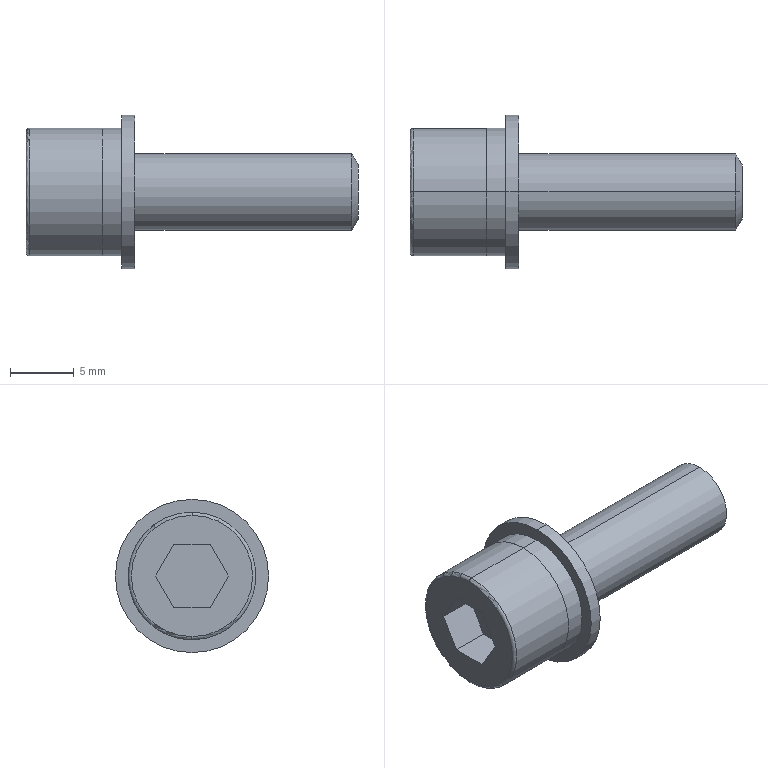Part | SolidWorks | features BaseBody 3 | 3 solids | 36 faces | box 26 x 12 x 12 mm | volume 1103 mm3 | plane 16 | cylinder 14 | torus 4 | cone 2 | commonest cylinder face diameters 7 x5 10 x5 6 x2 12 x2
STEP:
#1=CARTESIAN_POINT('',(26.,0.,2.134));
#2=VERTEX_POINT('',#1);
#3=CARTESIAN_POINT('',(26.,0.,-2.134));
#4=VERTEX_POINT('',#3);
#5=CARTESIAN_POINT('',(26.,0.,0.));
#6=DIRECTION('',(-1.,0.,0.));
#7=DIRECTION('',(0.,0.,1.));
#8=AXIS2_PLACEMENT_3D('',#5,#6,#7);
#9=CIRCLE('',#8,2.134);
#10=EDGE_CURVE('',#2,#4,#9,.T.);
#11=ORIENTED_EDGE('',*,*,#10,.T.);
#12=CARTESIAN_POINT('',(25.5,0.,-3.));
#13=VERTEX_POINT('',#12);
#14=CARTESIAN_POINT('',(25.5,0.,-3.));
#15=DIRECTION('',(-0.5,0.,-0.866));
#16=VECTOR('',#15,1000.);
#17=LINE('',#14,#16);
#18=EDGE_CURVE('',#4,#13,#17,.T.);
#19=ORIENTED_EDGE('',*,*,#18,.T.);
#20=CARTESIAN_POINT('',(25.5,0.,3.));
#21=VERTEX_POINT('',#20);
#22=CARTESIAN_POINT('',(25.5,0.,0.));
#23=DIRECTION('',(-1.,0.,0.));
#24=DIRECTION('',(0.,0.,1.));
#25=AXIS2_PLACEMENT_3D('',#22,#23,#24);
#26=CIRCLE('',#25,3.);
#27=EDGE_CURVE('',#21,#13,#26,.T.);
#28=ORIENTED_EDGE('',*,*,#27,.F.);
#29=CARTESIAN_POINT('',(25.5,0.,3.));
#30=DIRECTION('',(-0.5,0.,0.866));
#31=VECTOR('',#30,1000.);
#32=LINE('',#29,#31);
#33=EDGE_CURVE('',#2,#21,#32,.T.);
#34=ORIENTED_EDGE('',*,*,#33,.F.);
#35=EDGE_LOOP('',(#11,#19,#28,#34));
#36=FACE_OUTER_BOUND('',#35,.T.);
#37=CARTESIAN_POINT('',(25.5,0.,0.));
#38=DIRECTION('',(-1.,0.,0.));
#39=DIRECTION('',(0.,0.,1.));
#40=AXIS2_PLACEMENT_3D('',#37,#38,#39);
#41=CONICAL_SURFACE('',#40,3.,1.047);
#42=ADVANCED_FACE('',(#36),#41,.T.);
#43=CARTESIAN_POINT('',(0.25,0.,-5.));
#44=VERTEX_POINT('',#43);
#45=CARTESIAN_POINT('',(0.25,0.,5.));
#46=VERTEX_POINT('',#45);
#47=CARTESIAN_POINT('',(0.25,0.,0.));
#48=DIRECTION('',(1.,0.,0.));
#49=DIRECTION('',(0.,0.,1.));
#50=AXIS2_PLACEMENT_3D('',#47,#48,#49);
#51=CIRCLE('',#50,5.);
#52=EDGE_CURVE('',#44,#46,#51,.T.);
#53=ORIENTED_EDGE('',*,*,#52,.F.);
#54=CARTESIAN_POINT('',(0.,0.,-4.75));
#55=VERTEX_POINT('',#54);
#56=CARTESIAN_POINT('',(0.25,0.,-4.75));
#57=DIRECTION('',(0.,1.,0.));
#58=DIRECTION('',(0.,0.,1.));
#59=AXIS2_PLACEMENT_3D('',#56,#57,#58);
#60=CIRCLE('',#59,0.25);
#61=EDGE_CURVE('',#44,#55,#60,.T.);
#62=ORIENTED_EDGE('',*,*,#61,.T.);
#63=CARTESIAN_POINT('',(0.,0.,4.75));
#64=VERTEX_POINT('',#63);
#65=CARTESIAN_POINT('',(0.,0.,0.));
#66=DIRECTION('',(-1.,0.,0.));
#67=DIRECTION('',(0.,0.,1.));
#68=AXIS2_PLACEMENT_3D('',#65,#66,#67);
#69=CIRCLE('',#68,4.75);
#70=EDGE_CURVE('',#64,#55,#69,.T.);
#71=ORIENTED_EDGE('',*,*,#70,.F.);
#72=CARTESIAN_POINT('',(0.25,0.,4.75));
#73=DIRECTION('',(0.,-1.,0.));
#74=DIRECTION('',(0.,0.,-1.));
#75=AXIS2_PLACEMENT_3D('',#72,#73,#74);
#76=CIRCLE('',#75,0.25);
#77=EDGE_CURVE('',#46,#64,#76,.T.);
#78=ORIENTED_EDGE('',*,*,#77,.F.);
#79=EDGE_LOOP('',(#53,#62,#71,#78));
#80=FACE_OUTER_BOUND('',#79,.T.);
#81=CARTESIAN_POINT('',(0.25,0.,0.));
#82=DIRECTION('',(-1.,0.,0.));
#83=DIRECTION('',(0.,0.,1.));
#84=AXIS2_PLACEMENT_3D('',#81,#82,#83);
#85=TOROIDAL_SURFACE('',#84,4.75,0.25);
#86=ADVANCED_FACE('',(#80),#85,.T.);
#87=CARTESIAN_POINT('',(6.25,0.,3.));
#88=VERTEX_POINT('',#87);
#89=CARTESIAN_POINT('',(6.25,0.,-3.));
#90=VERTEX_POINT('',#89);
#91=CARTESIAN_POINT('',(6.25,0.,0.));
#92=DIRECTION('',(1.,0.,0.));
#93=DIRECTION('',(0.,0.,-1.));
#94=AXIS2_PLACEMENT_3D('',#91,#92,#93);
#95=CIRCLE('',#94,3.);
#96=EDGE_CURVE('',#88,#90,#95,.T.);
#97=ORIENTED_EDGE('',*,*,#96,.F.);
#98=CARTESIAN_POINT('',(6.,0.,3.25));
#99=VERTEX_POINT('',#98);
#100=CARTESIAN_POINT('',(6.25,0.,3.25));
#101=DIRECTION('',(0.,1.,0.));
#102=DIRECTION('',(0.,0.,1.));
#103=AXIS2_PLACEMENT_3D('',#100,#101,#102);
#104=CIRCLE('',#103,0.25);
#105=EDGE_CURVE('',#88,#99,#104,.T.);
#106=ORIENTED_EDGE('',*,*,#105,.T.);
#107=CARTESIAN_POINT('',(6.,0.,-3.25));
#108=VERTEX_POINT('',#107);
#109=CARTESIAN_POINT('',(6.,0.,0.));
#110=DIRECTION('',(1.,0.,0.));
#111=DIRECTION('',(0.,0.,-1.));
#112=AXIS2_PLACEMENT_3D('',#109,#110,#111);
#113=CIRCLE('',#112,3.25);
#114=EDGE_CURVE('',#99,#108,#113,.T.);
#115=ORIENTED_EDGE('',*,*,#114,.T.);
#116=CARTESIAN_POINT('',(6.25,0.,-3.25));
#117=DIRECTION('',(0.,-1.,0.));
#118=DIRECTION('',(0.,0.,-1.));
#119=AXIS2_PLACEMENT_3D('',#116,#117,#118);
#120=CIRCLE('',#119,0.25);
#121=EDGE_CURVE('',#90,#108,#120,.T.);
#122=ORIENTED_EDGE('',*,*,#121,.F.);
#123=EDGE_LOOP('',(#97,#106,#115,#122));
#124=FACE_OUTER_BOUND('',#123,.T.);
#125=CARTESIAN_POINT('',(6.25,0.,0.));
#126=DIRECTION('',(1.,0.,0.));
#127=DIRECTION('',(0.,0.,-1.));
#128=AXIS2_PLACEMENT_3D('',#125,#126,#127);
#129=TOROIDAL_SURFACE('',#128,3.25,0.25);
#130=ADVANCED_FACE('',(#124),#129,.F.);
#131=ORIENTED_EDGE('',*,*,#52,.T.);
#132=CARTESIAN_POINT('',(6.,0.,5.));
#133=VERTEX_POINT('',#132);
#134=CARTESIAN_POINT('',(0.,0.,5.));
#135=DIRECTION('',(1.,0.,0.));
#136=VECTOR('',#135,1000.);
#137=LINE('',#134,#136);
#138=EDGE_CURVE('',#46,#133,#137,.T.);
#139=ORIENTED_EDGE('',*,*,#138,.T.);
#140=CARTESIAN_POINT('',(6.,0.,-5.));
#141=VERTEX_POINT('',#140);
#142=CARTESIAN_POINT('',(6.,0.,0.));
#143=DIRECTION('',(1.,0.,0.));
#144=DIRECTION('',(0.,0.,-1.));
#145=AXIS2_PLACEMENT_3D('',#142,#143,#144);
#146=CIRCLE('',#145,5.);
#147=EDGE_CURVE('',#141,#133,#146,.T.);
#148=ORIENTED_EDGE('',*,*,#147,.F.);
#149=CARTESIAN_POINT('',(0.,0.,-5.));
#150=DIRECTION('',(1.,0.,0.));
#151=VECTOR('',#150,1000.);
#152=LINE('',#149,#151);
#153=EDGE_CURVE('',#44,#141,#152,.T.);
#154=ORIENTED_EDGE('',*,*,#153,.F.);
#155=EDGE_LOOP('',(#131,#139,#148,#154));
#156=FACE_OUTER_BOUND('',#155,.T.);
#157=CARTESIAN_POINT('',(0.,0.,0.));
#158=DIRECTION('',(1.,0.,0.));
#159=DIRECTION('',(0.,0.,-1.));
#160=AXIS2_PLACEMENT_3D('',#157,#158,#159);
#161=CYLINDRICAL_SURFACE('',#160,5.);
#162=ADVANCED_FACE('',(#156),#161,.T.);
#163=CARTESIAN_POINT('',(6.25,0.,0.));
#164=DIRECTION('',(1.,0.,0.));
#165=DIRECTION('',(0.,0.,-1.));
#166=AXIS2_PLACEMENT_3D('',#163,#164,#165);
#167=CIRCLE('',#166,3.);
#168=EDGE_CURVE('',#90,#88,#167,.T.);
#169=ORIENTED_EDGE('',*,*,#168,.T.);
#170=CARTESIAN_POINT('',(0.,0.,3.));
#171=DIRECTION('',(1.,0.,0.));
#172=VECTOR('',#171,1000.);
#173=LINE('',#170,#172);
#174=EDGE_CURVE('',#88,#21,#173,.T.);
#175=ORIENTED_EDGE('',*,*,#174,.T.);
#176=ORIENTED_EDGE('',*,*,#27,.T.);
#177=CARTESIAN_POINT('',(0.,0.,-3.));
#178=DIRECTION('',(1.,0.,0.));
#179=VECTOR('',#178,1000.);
#180=LINE('',#177,#179);
#181=EDGE_CURVE('',#90,#13,#180,.T.);
#182=ORIENTED_EDGE('',*,*,#181,.F.);
#183=EDGE_LOOP('',(#169,#175,#176,#182));
#184=FACE_OUTER_BOUND('',#183,.T.);
#185=CARTESIAN_POINT('',(0.,0.,0.));
#186=DIRECTION('',(1.,0.,0.));
#187=DIRECTION('',(0.,0.,-1.));
#188=AXIS2_PLACEMENT_3D('',#185,#186,#187);
#189=CYLINDRICAL_SURFACE('',#188,3.);
#190=ADVANCED_FACE('',(#184),#189,.T.);
#191=ORIENTED_EDGE('',*,*,#174,.F.);
#192=ORIENTED_EDGE('',*,*,#96,.T.);
#193=ORIENTED_EDGE('',*,*,#181,.T.);
#194=CARTESIAN_POINT('',(25.5,0.,0.));
#195=DIRECTION('',(-1.,0.,0.));
#196=DIRECTION('',(0.,0.,1.));
#197=AXIS2_PLACEMENT_3D('',#194,#195,#196);
#198=CIRCLE('',#197,3.);
#199=EDGE_CURVE('',#13,#21,#198,.T.);
#200=ORIENTED_EDGE('',*,*,#199,.T.);
#201=EDGE_LOOP('',(#191,#192,#193,#200));
#202=FACE_OUTER_BOUND('',#201,.T.);
#203=CARTESIAN_POINT('',(0.,0.,0.));
#204=DIRECTION('',(1.,0.,0.));
#205=DIRECTION('',(0.,0.,-1.));
#206=AXIS2_PLACEMENT_3D('',#203,#204,#205);
#207=CYLINDRICAL_SURFACE('',#206,3.);
#208=ADVANCED_FACE('',(#202),#207,.T.);
#209=ORIENTED_EDGE('',*,*,#70,.T.);
#210=CARTESIAN_POINT('',(0.,0.,0.));
#211=DIRECTION('',(-1.,0.,0.));
#212=DIRECTION('',(0.,0.,1.));
#213=AXIS2_PLACEMENT_3D('',#210,#211,#212);
#214=CIRCLE('',#213,4.75);
#215=EDGE_CURVE('',#55,#64,#214,.T.);
#216=ORIENTED_EDGE('',*,*,#215,.T.);
#217=EDGE_LOOP('',(#209,#216));
#218=FACE_OUTER_BOUND('',#217,.T.);
#219=CARTESIAN_POINT('',(0.,-2.86,0.));
#220=VERTEX_POINT('',#219);
#221=CARTESIAN_POINT('',(0.,-1.43,2.477));
#222=VERTEX_POINT('',#221);
#223=CARTESIAN_POINT('',(0.,-2.86,0.));
#224=DIRECTION('',(0.,0.5,0.866));
#225=VECTOR('',#224,1000.);
#226=LINE('',#223,#225);
#227=EDGE_CURVE('',#220,#222,#226,.T.);
#228=ORIENTED_EDGE('',*,*,#227,.F.);
#229=CARTESIAN_POINT('',(0.,-1.43,-2.477));
#230=VERTEX_POINT('',#229);
#231=CARTESIAN_POINT('',(0.,-1.43,-2.477));
#232=DIRECTION('',(0.,-0.5,0.866));
#233=VECTOR('',#232,1000.);
#234=LINE('',#231,#233);
#235=EDGE_CURVE('',#230,#220,#234,.T.);
#236=ORIENTED_EDGE('',*,*,#235,.F.);
#237=CARTESIAN_POINT('',(0.,1.43,-2.477));
#238=VERTEX_POINT('',#237);
#239=CARTESIAN_POINT('',(0.,1.43,-2.477));
#240=DIRECTION('',(0.,-1.,0.));
#241=VECTOR('',#240,1000.);
#242=LINE('',#239,#241);
#243=EDGE_CURVE('',#238,#230,#242,.T.);
#244=ORIENTED_EDGE('',*,*,#243,.F.);
#245=CARTESIAN_POINT('',(0.,2.86,0.));
#246=VERTEX_POINT('',#245);
#247=CARTESIAN_POINT('',(0.,2.86,0.));
#248=DIRECTION('',(0.,-0.5,-0.866));
#249=VECTOR('',#248,1000.);
#250=LINE('',#247,#249);
#251=EDGE_CURVE('',#246,#238,#250,.T.);
#252=ORIENTED_EDGE('',*,*,#251,.F.);
#253=CARTESIAN_POINT('',(0.,1.43,2.477));
#254=VERTEX_POINT('',#253);
#255=CARTESIAN_POINT('',(0.,1.43,2.477));
#256=DIRECTION('',(0.,0.5,-0.866));
#257=VECTOR('',#256,1000.);
#258=LINE('',#255,#257);
#259=EDGE_CURVE('',#254,#246,#258,.T.);
#260=ORIENTED_EDGE('',*,*,#259,.F.);
#261=CARTESIAN_POINT('',(0.,-1.43,2.477));
#262=DIRECTION('',(0.,1.,0.));
#263=VECTOR('',#262,1000.);
#264=LINE('',#261,#263);
#265=EDGE_CURVE('',#222,#254,#264,.T.);
#266=ORIENTED_EDGE('',*,*,#265,.F.);
#267=EDGE_LOOP('',(#228,#236,#244,#252,#260,#266));
#268=FACE_BOUND('',#267,.T.);
#269=CARTESIAN_POINT('',(0.,0.,0.));
#270=DIRECTION('',(-1.,0.,0.));
#271=DIRECTION('',(0.,0.,1.));
#272=AXIS2_PLACEMENT_3D('',#269,#270,#271);
#273=PLANE('',#272);
#274=ADVANCED_FACE('',(#218,#268),#273,.T.);
#275=ORIENTED_EDGE('',*,*,#138,.F.);
#276=CARTESIAN_POINT('',(0.25,0.,0.));
#277=DIRECTION('',(1.,0.,0.));
#278=DIRECTION('',(0.,0.,1.));
#279=AXIS2_PLACEMENT_3D('',#276,#277,#278);
#280=CIRCLE('',#279,5.);
#281=EDGE_CURVE('',#46,#44,#280,.T.);
#282=ORIENTED_EDGE('',*,*,#281,.T.);
#283=ORIENTED_EDGE('',*,*,#153,.T.);
#284=CARTESIAN_POINT('',(6.,0.,0.));
#285=DIRECTION('',(1.,0.,0.));
#286=DIRECTION('',(0.,0.,-1.));
#287=AXIS2_PLACEMENT_3D('',#284,#285,#286);
#288=CIRCLE('',#287,5.);
#289=EDGE_CURVE('',#133,#141,#288,.T.);
#290=ORIENTED_EDGE('',*,*,#289,.F.);
#291=EDGE_LOOP('',(#275,#282,#283,#290));
#292=FACE_OUTER_BOUND('',#291,.T.);
#293=CARTESIAN_POINT('',(0.,0.,0.));
#294=DIRECTION('',(1.,0.,0.));
#295=DIRECTION('',(0.,0.,-1.));
#296=AXIS2_PLACEMENT_3D('',#293,#294,#295);
#297=CYLINDRICAL_SURFACE('',#296,5.);
#298=ADVANCED_FACE('',(#292),#297,.T.);
#299=ORIENTED_EDGE('',*,*,#147,.T.);
#300=ORIENTED_EDGE('',*,*,#289,.T.);
#301=EDGE_LOOP('',(#299,#300));
#302=FACE_OUTER_BOUND('',#301,.T.);
#303=CARTESIAN_POINT('',(6.,0.,0.));
#304=DIRECTION('',(1.,0.,0.));
#305=DIRECTION('',(0.,0.,-1.));
#306=AXIS2_PLACEMENT_3D('',#303,#304,#305);
#307=CIRCLE('',#306,3.25);
#308=EDGE_CURVE('',#108,#99,#307,.T.);
#309=ORIENTED_EDGE('',*,*,#308,.F.);
#310=ORIENTED_EDGE('',*,*,#114,.F.);
#311=EDGE_LOOP('',(#309,#310));
#312=FACE_BOUND('',#311,.T.);
#313=CARTESIAN_POINT('',(6.,5.,0.));
#314=DIRECTION('',(1.,0.,0.));
#315=DIRECTION('',(0.,0.,-1.));
#316=AXIS2_PLACEMENT_3D('',#313,#314,#315);
#317=PLANE('',#316);
#318=ADVANCED_FACE('',(#302,#312),#317,.T.);
#319=ORIENTED_EDGE('',*,*,#105,.F.);
#320=ORIENTED_EDGE('',*,*,#168,.F.);
#321=ORIENTED_EDGE('',*,*,#121,.T.);
#322=ORIENTED_EDGE('',*,*,#308,.T.);
#323=EDGE_LOOP('',(#319,#320,#321,#322));
#324=FACE_OUTER_BOUND('',#323,.T.);
#325=CARTESIAN_POINT('',(6.25,0.,0.));
#326=DIRECTION('',(1.,0.,0.));
#327=DIRECTION('',(0.,0.,-1.));
#328=AXIS2_PLACEMENT_3D('',#325,#326,#327);
#329=TOROIDAL_SURFACE('',#328,3.25,0.25);
#330=ADVANCED_FACE('',(#324),#329,.F.);
#331=ORIENTED_EDGE('',*,*,#227,.T.);
#332=CARTESIAN_POINT('',(3.,-1.43,2.477));
#333=VERTEX_POINT('',#332);
#334=CARTESIAN_POINT('',(3.,-1.43,2.477));
#335=DIRECTION('',(-1.,0.,0.));
#336=VECTOR('',#335,1000.);
#337=LINE('',#334,#336);
#338=EDGE_CURVE('',#333,#222,#337,.T.);
#339=ORIENTED_EDGE('',*,*,#338,.F.);
#340=CARTESIAN_POINT('',(3.,-2.86,0.));
#341=VERTEX_POINT('',#340);
#342=CARTESIAN_POINT('',(3.,-2.86,0.));
#343=DIRECTION('',(0.,0.5,0.866));
#344=VECTOR('',#343,1000.);
#345=LINE('',#342,#344);
#346=EDGE_CURVE('',#341,#333,#345,.T.);
#347=ORIENTED_EDGE('',*,*,#346,.F.);
#348=CARTESIAN_POINT('',(3.,-2.86,0.));
#349=DIRECTION('',(-1.,0.,0.));
#350=VECTOR('',#349,1000.);
#351=LINE('',#348,#350);
#352=EDGE_CURVE('',#341,#220,#351,.T.);
#353=ORIENTED_EDGE('',*,*,#352,.T.);
#354=EDGE_LOOP('',(#331,#339,#347,#353));
#355=FACE_OUTER_BOUND('',#354,.T.);
#356=CARTESIAN_POINT('',(3.,-2.86,0.));
#357=DIRECTION('',(0.,-0.866,0.5));
#358=DIRECTION('',(0.,-0.5,-0.866));
#359=AXIS2_PLACEMENT_3D('',#356,#357,#358);
#360=PLANE('',#359);
#361=ADVANCED_FACE('',(#355),#360,.F.);
#362=ORIENTED_EDGE('',*,*,#235,.T.);
#363=ORIENTED_EDGE('',*,*,#352,.F.);
#364=CARTESIAN_POINT('',(3.,-1.43,-2.477));
#365=VERTEX_POINT('',#364);
#366=CARTESIAN_POINT('',(3.,-1.43,-2.477));
#367=DIRECTION('',(0.,-0.5,0.866));
#368=VECTOR('',#367,1000.);
#369=LINE('',#366,#368);
#370=EDGE_CURVE('',#365,#341,#369,.T.);
#371=ORIENTED_EDGE('',*,*,#370,.F.);
#372=CARTESIAN_POINT('',(3.,-1.43,-2.477));
#373=DIRECTION('',(-1.,0.,0.));
#374=VECTOR('',#373,1000.);
#375=LINE('',#372,#374);
#376=EDGE_CURVE('',#365,#230,#375,.T.);
#377=ORIENTED_EDGE('',*,*,#376,.T.);
#378=EDGE_LOOP('',(#362,#363,#371,#377));
#379=FACE_OUTER_BOUND('',#378,.T.);
#380=CARTESIAN_POINT('',(3.,-1.43,-2.477));
#381=DIRECTION('',(0.,-0.866,-0.5));
#382=DIRECTION('',(0.,0.5,-0.866));
#383=AXIS2_PLACEMENT_3D('',#380,#381,#382);
#384=PLANE('',#383);
#385=ADVANCED_FACE('',(#379),#384,.F.);
#386=ORIENTED_EDGE('',*,*,#243,.T.);
#387=ORIENTED_EDGE('',*,*,#376,.F.);
#388=CARTESIAN_POINT('',(3.,1.43,-2.477));
#389=VERTEX_POINT('',#388);
#390=CARTESIAN_POINT('',(3.,1.43,-2.477));
#391=DIRECTION('',(0.,-1.,0.));
#392=VECTOR('',#391,1000.);
#393=LINE('',#390,#392);
#394=EDGE_CURVE('',#389,#365,#393,.T.);
#395=ORIENTED_EDGE('',*,*,#394,.F.);
#396=CARTESIAN_POINT('',(3.,1.43,-2.477));
#397=DIRECTION('',(-1.,0.,0.));
#398=VECTOR('',#397,1000.);
#399=LINE('',#396,#398);
#400=EDGE_CURVE('',#389,#238,#399,.T.);
#401=ORIENTED_EDGE('',*,*,#400,.T.);
#402=EDGE_LOOP('',(#386,#387,#395,#401));
#403=FACE_OUTER_BOUND('',#402,.T.);
#404=CARTESIAN_POINT('',(3.,1.43,-2.477));
#405=DIRECTION('',(0.,0.,-1.));
#406=DIRECTION('',(-1.,0.,0.));
#407=AXIS2_PLACEMENT_3D('',#404,#405,#406);
#408=PLANE('',#407);
#409=ADVANCED_FACE('',(#403),#408,.F.);
#410=ORIENTED_EDGE('',*,*,#251,.T.);
#411=ORIENTED_EDGE('',*,*,#400,.F.);
#412=CARTESIAN_POINT('',(3.,2.86,0.));
#413=VERTEX_POINT('',#412);
#414=CARTESIAN_POINT('',(3.,2.86,0.));
#415=DIRECTION('',(0.,-0.5,-0.866));
#416=VECTOR('',#415,1000.);
#417=LINE('',#414,#416);
#418=EDGE_CURVE('',#413,#389,#417,.T.);
#419=ORIENTED_EDGE('',*,*,#418,.F.);
#420=CARTESIAN_POINT('',(3.,2.86,0.));
#421=DIRECTION('',(-1.,0.,0.));
#422=VECTOR('',#421,1000.);
#423=LINE('',#420,#422);
#424=EDGE_CURVE('',#413,#246,#423,.T.);
#425=ORIENTED_EDGE('',*,*,#424,.T.);
#426=EDGE_LOOP('',(#410,#411,#419,#425));
#427=FACE_OUTER_BOUND('',#426,.T.);
#428=CARTESIAN_POINT('',(3.,2.86,0.));
#429=DIRECTION('',(0.,0.866,-0.5));
#430=DIRECTION('',(0.,0.5,0.866));
#431=AXIS2_PLACEMENT_3D('',#428,#429,#430);
#432=PLANE('',#431);
#433=ADVANCED_FACE('',(#427),#432,.F.);
#434=ORIENTED_EDGE('',*,*,#259,.T.);
#435=ORIENTED_EDGE('',*,*,#424,.F.);
#436=CARTESIAN_POINT('',(3.,1.43,2.477));
#437=VERTEX_POINT('',#436);
#438=CARTESIAN_POINT('',(3.,1.43,2.477));
#439=DIRECTION('',(0.,0.5,-0.866));
#440=VECTOR('',#439,1000.);
#441=LINE('',#438,#440);
#442=EDGE_CURVE('',#437,#413,#441,.T.);
#443=ORIENTED_EDGE('',*,*,#442,.F.);
#444=CARTESIAN_POINT('',(3.,1.43,2.477));
#445=DIRECTION('',(-1.,0.,0.));
#446=VECTOR('',#445,1000.);
#447=LINE('',#444,#446);
#448=EDGE_CURVE('',#437,#254,#447,.T.);
#449=ORIENTED_EDGE('',*,*,#448,.T.);
#450=EDGE_LOOP('',(#434,#435,#443,#449));
#451=FACE_OUTER_BOUND('',#450,.T.);
#452=CARTESIAN_POINT('',(3.,1.43,2.477));
#453=DIRECTION('',(0.,0.866,0.5));
#454=DIRECTION('',(0.,-0.5,0.866));
#455=AXIS2_PLACEMENT_3D('',#452,#453,#454);
#456=PLANE('',#455);
#457=ADVANCED_FACE('',(#451),#456,.F.);
#458=ORIENTED_EDGE('',*,*,#265,.T.);
#459=ORIENTED_EDGE('',*,*,#448,.F.);
#460=CARTESIAN_POINT('',(3.,-1.43,2.477));
#461=DIRECTION('',(0.,1.,0.));
#462=VECTOR('',#461,1000.);
#463=LINE('',#460,#462);
#464=EDGE_CURVE('',#333,#437,#463,.T.);
#465=ORIENTED_EDGE('',*,*,#464,.F.);
#466=ORIENTED_EDGE('',*,*,#338,.T.);
#467=EDGE_LOOP('',(#458,#459,#465,#466));
#468=FACE_OUTER_BOUND('',#467,.T.);
#469=CARTESIAN_POINT('',(3.,-1.43,2.477));
#470=DIRECTION('',(0.,0.,1.));
#471=DIRECTION('',(0.,-1.,0.));
#472=AXIS2_PLACEMENT_3D('',#469,#470,#471);
#473=PLANE('',#472);
#474=ADVANCED_FACE('',(#468),#473,.F.);
#475=ORIENTED_EDGE('',*,*,#346,.T.);
#476=ORIENTED_EDGE('',*,*,#464,.T.);
#477=ORIENTED_EDGE('',*,*,#442,.T.);
#478=ORIENTED_EDGE('',*,*,#418,.T.);
#479=ORIENTED_EDGE('',*,*,#394,.T.);
#480=ORIENTED_EDGE('',*,*,#370,.T.);
#481=EDGE_LOOP('',(#475,#476,#477,#478,#479,#480));
#482=FACE_OUTER_BOUND('',#481,.T.);
#483=CARTESIAN_POINT('',(3.,-1.43,2.477));
#484=DIRECTION('',(-1.,0.,0.));
#485=DIRECTION('',(0.,0.,1.));
#486=AXIS2_PLACEMENT_3D('',#483,#484,#485);
#487=PLANE('',#486);
#488=ADVANCED_FACE('',(#482),#487,.T.);
#489=ORIENTED_EDGE('',*,*,#61,.F.);
#490=ORIENTED_EDGE('',*,*,#281,.F.);
#491=ORIENTED_EDGE('',*,*,#77,.T.);
#492=ORIENTED_EDGE('',*,*,#215,.F.);
#493=EDGE_LOOP('',(#489,#490,#491,#492));
#494=FACE_OUTER_BOUND('',#493,.T.);
#495=CARTESIAN_POINT('',(0.25,0.,0.));
#496=DIRECTION('',(-1.,0.,0.));
#497=DIRECTION('',(0.,0.,1.));
#498=AXIS2_PLACEMENT_3D('',#495,#496,#497);
#499=TOROIDAL_SURFACE('',#498,4.75,0.25);
#500=ADVANCED_FACE('',(#494),#499,.T.);
#501=ORIENTED_EDGE('',*,*,#18,.F.);
#502=CARTESIAN_POINT('',(26.,0.,0.));
#503=DIRECTION('',(-1.,0.,0.));
#504=DIRECTION('',(0.,0.,1.));
#505=AXIS2_PLACEMENT_3D('',#502,#503,#504);
#506=CIRCLE('',#505,2.134);
#507=EDGE_CURVE('',#4,#2,#506,.T.);
#508=ORIENTED_EDGE('',*,*,#507,.T.);
#509=ORIENTED_EDGE('',*,*,#33,.T.);
#510=ORIENTED_EDGE('',*,*,#199,.F.);
#511=EDGE_LOOP('',(#501,#508,#509,#510));
#512=FACE_OUTER_BOUND('',#511,.T.);
#513=CARTESIAN_POINT('',(25.5,0.,0.));
#514=DIRECTION('',(-1.,0.,0.));
#515=DIRECTION('',(0.,0.,1.));
#516=AXIS2_PLACEMENT_3D('',#513,#514,#515);
#517=CONICAL_SURFACE('',#516,3.,1.047);
#518=ADVANCED_FACE('',(#512),#517,.T.);
#519=ORIENTED_EDGE('',*,*,#10,.F.);
#520=ORIENTED_EDGE('',*,*,#507,.F.);
#521=EDGE_LOOP('',(#519,#520));
#522=FACE_OUTER_BOUND('',#521,.T.);
#523=CARTESIAN_POINT('',(26.,3.,0.));
#524=DIRECTION('',(1.,0.,0.));
#525=DIRECTION('',(0.,0.,-1.));
#526=AXIS2_PLACEMENT_3D('',#523,#524,#525);
#527=PLANE('',#526);
#528=ADVANCED_FACE('',(#522),#527,.T.);
#529=CLOSED_SHELL('',(#42,#86,#130,#162,#190,#208,#274,#298,#318,#330,#361,#385,#409,#433,#457,#474,#488,#500,#518,#528));
#530=MANIFOLD_SOLID_BREP('',#529);
#531=CARTESIAN_POINT('',(7.5,0.,-5.));
#532=VERTEX_POINT('',#531);
#533=CARTESIAN_POINT('',(7.5,4.913,-0.931));
#534=VERTEX_POINT('',#533);
#535=CARTESIAN_POINT('',(7.5,0.,0.));
#536=DIRECTION('',(1.,0.,0.));
#537=DIRECTION('',(0.,0.,-1.));
#538=AXIS2_PLACEMENT_3D('',#535,#536,#537);
#539=CIRCLE('',#538,5.);
#540=EDGE_CURVE('',#532,#534,#539,.T.);
#541=ORIENTED_EDGE('',*,*,#540,.F.);
#542=CARTESIAN_POINT('',(6.,0.,-5.));
#543=VERTEX_POINT('',#542);
#544=CARTESIAN_POINT('',(7.5,0.,-5.));
#545=DIRECTION('',(-1.,0.,0.));
#546=VECTOR('',#545,1000.);
#547=LINE('',#544,#546);
#548=EDGE_CURVE('',#532,#543,#547,.T.);
#549=ORIENTED_EDGE('',*,*,#548,.T.);
#550=CARTESIAN_POINT('',(6.,4.913,-0.931));
#551=VERTEX_POINT('',#550);
#552=CARTESIAN_POINT('',(6.,0.,0.));
#553=DIRECTION('',(1.,0.,0.));
#554=DIRECTION('',(0.,0.,-1.));
#555=AXIS2_PLACEMENT_3D('',#552,#553,#554);
#556=CIRCLE('',#555,5.);
#557=EDGE_CURVE('',#543,#551,#556,.T.);
#558=ORIENTED_EDGE('',*,*,#557,.T.);
#559=CARTESIAN_POINT('',(7.5,4.913,-0.931));
#560=DIRECTION('',(-1.,0.,0.));
#561=VECTOR('',#560,1000.);
#562=LINE('',#559,#561);
#563=EDGE_CURVE('',#534,#551,#562,.T.);
#564=ORIENTED_EDGE('',*,*,#563,.F.);
#565=EDGE_LOOP('',(#541,#549,#558,#564));
#566=FACE_OUTER_BOUND('',#565,.T.);
#567=CARTESIAN_POINT('',(7.5,0.,0.));
#568=DIRECTION('',(-1.,0.,0.));
#569=DIRECTION('',(0.,0.,1.));
#570=AXIS2_PLACEMENT_3D('',#567,#568,#569);
#571=CYLINDRICAL_SURFACE('',#570,5.);
#572=ADVANCED_FACE('',(#566),#571,.T.);
#573=ORIENTED_EDGE('',*,*,#548,.F.);
#574=CARTESIAN_POINT('',(7.5,0.,5.));
#575=VERTEX_POINT('',#574);
#576=CARTESIAN_POINT('',(7.5,0.,0.));
#577=DIRECTION('',(1.,0.,0.));
#578=DIRECTION('',(0.,0.,-1.));
#579=AXIS2_PLACEMENT_3D('',#576,#577,#578);
#580=CIRCLE('',#579,5.);
#581=EDGE_CURVE('',#575,#532,#580,.T.);
#582=ORIENTED_EDGE('',*,*,#581,.F.);
#583=CARTESIAN_POINT('',(6.,0.,5.));
#584=VERTEX_POINT('',#583);
#585=CARTESIAN_POINT('',(7.5,0.,5.));
#586=DIRECTION('',(-1.,0.,0.));
#587=VECTOR('',#586,1000.);
#588=LINE('',#585,#587);
#589=EDGE_CURVE('',#575,#584,#588,.T.);
#590=ORIENTED_EDGE('',*,*,#589,.T.);
#591=CARTESIAN_POINT('',(6.,0.,0.));
#592=DIRECTION('',(1.,0.,0.));
#593=DIRECTION('',(0.,0.,-1.));
#594=AXIS2_PLACEMENT_3D('',#591,#592,#593);
#595=CIRCLE('',#594,5.);
#596=EDGE_CURVE('',#584,#543,#595,.T.);
#597=ORIENTED_EDGE('',*,*,#596,.T.);
#598=EDGE_LOOP('',(#573,#582,#590,#597));
#599=FACE_OUTER_BOUND('',#598,.T.);
#600=CARTESIAN_POINT('',(7.5,0.,0.));
#601=DIRECTION('',(-1.,0.,0.));
#602=DIRECTION('',(0.,0.,1.));
#603=AXIS2_PLACEMENT_3D('',#600,#601,#602);
#604=CYLINDRICAL_SURFACE('',#603,5.);
#605=ADVANCED_FACE('',(#599),#604,.T.);
#606=CARTESIAN_POINT('',(7.5,0.,-3.5));
#607=VERTEX_POINT('',#606);
#608=CARTESIAN_POINT('',(7.5,0.,3.5));
#609=VERTEX_POINT('',#608);
#610=CARTESIAN_POINT('',(7.5,0.,0.));
#611=DIRECTION('',(-1.,0.,0.));
#612=DIRECTION('',(0.,0.,-1.));
#613=AXIS2_PLACEMENT_3D('',#610,#611,#612);
#614=CIRCLE('',#613,3.5);
#615=EDGE_CURVE('',#607,#609,#614,.T.);
#616=ORIENTED_EDGE('',*,*,#615,.F.);
#617=CARTESIAN_POINT('',(6.,0.,-3.5));
#618=VERTEX_POINT('',#617);
#619=CARTESIAN_POINT('',(7.5,0.,-3.5));
#620=DIRECTION('',(-1.,0.,0.));
#621=VECTOR('',#620,1000.);
#622=LINE('',#619,#621);
#623=EDGE_CURVE('',#607,#618,#622,.T.);
#624=ORIENTED_EDGE('',*,*,#623,.T.);
#625=CARTESIAN_POINT('',(6.,0.,3.5));
#626=VERTEX_POINT('',#625);
#627=CARTESIAN_POINT('',(6.,0.,0.));
#628=DIRECTION('',(-1.,0.,0.));
#629=DIRECTION('',(0.,0.,-1.));
#630=AXIS2_PLACEMENT_3D('',#627,#628,#629);
#631=CIRCLE('',#630,3.5);
#632=EDGE_CURVE('',#618,#626,#631,.T.);
#633=ORIENTED_EDGE('',*,*,#632,.T.);
#634=CARTESIAN_POINT('',(7.5,0.,3.5));
#635=DIRECTION('',(-1.,0.,0.));
#636=VECTOR('',#635,1000.);
#637=LINE('',#634,#636);
#638=EDGE_CURVE('',#609,#626,#637,.T.);
#639=ORIENTED_EDGE('',*,*,#638,.F.);
#640=EDGE_LOOP('',(#616,#624,#633,#639));
#641=FACE_OUTER_BOUND('',#640,.T.);
#642=CARTESIAN_POINT('',(7.5,0.,0.));
#643=DIRECTION('',(-1.,0.,0.));
#644=DIRECTION('',(0.,0.,1.));
#645=AXIS2_PLACEMENT_3D('',#642,#643,#644);
#646=CYLINDRICAL_SURFACE('',#645,3.5);
#647=ADVANCED_FACE('',(#641),#646,.F.);
#648=CARTESIAN_POINT('',(7.5,3.498,0.1166));
#649=VERTEX_POINT('',#648);
#650=CARTESIAN_POINT('',(7.5,0.,0.));
#651=DIRECTION('',(-1.,0.,0.));
#652=DIRECTION('',(0.,0.,-1.));
#653=AXIS2_PLACEMENT_3D('',#650,#651,#652);
#654=CIRCLE('',#653,3.5);
#655=EDGE_CURVE('',#609,#649,#654,.T.);
#656=ORIENTED_EDGE('',*,*,#655,.F.);
#657=ORIENTED_EDGE('',*,*,#638,.T.);
#658=CARTESIAN_POINT('',(6.,3.498,0.1166));
#659=VERTEX_POINT('',#658);
#660=CARTESIAN_POINT('',(6.,0.,0.));
#661=DIRECTION('',(-1.,0.,0.));
#662=DIRECTION('',(0.,0.,-1.));
#663=AXIS2_PLACEMENT_3D('',#660,#661,#662);
#664=CIRCLE('',#663,3.5);
#665=EDGE_CURVE('',#626,#659,#664,.T.);
#666=ORIENTED_EDGE('',*,*,#665,.T.);
#667=CARTESIAN_POINT('',(7.5,3.498,0.1166));
#668=DIRECTION('',(-1.,0.,0.));
#669=VECTOR('',#668,1000.);
#670=LINE('',#667,#669);
#671=EDGE_CURVE('',#649,#659,#670,.T.);
#672=ORIENTED_EDGE('',*,*,#671,.F.);
#673=EDGE_LOOP('',(#656,#657,#666,#672));
#674=FACE_OUTER_BOUND('',#673,.T.);
#675=CARTESIAN_POINT('',(7.5,0.,0.));
#676=DIRECTION('',(-1.,0.,0.));
#677=DIRECTION('',(0.,0.,1.));
#678=AXIS2_PLACEMENT_3D('',#675,#676,#677);
#679=CYLINDRICAL_SURFACE('',#678,3.5);
#680=ADVANCED_FACE('',(#674),#679,.F.);
#681=ORIENTED_EDGE('',*,*,#623,.F.);
#682=CARTESIAN_POINT('',(7.5,3.498,-0.1144));
#683=VERTEX_POINT('',#682);
#684=CARTESIAN_POINT('',(7.5,0.,0.));
#685=DIRECTION('',(-1.,0.,0.));
#686=DIRECTION('',(0.,0.,-1.));
#687=AXIS2_PLACEMENT_3D('',#684,#685,#686);
#688=CIRCLE('',#687,3.5);
#689=EDGE_CURVE('',#683,#607,#688,.T.);
#690=ORIENTED_EDGE('',*,*,#689,.F.);
#691=CARTESIAN_POINT('',(6.,3.498,-0.1144));
#692=VERTEX_POINT('',#691);
#693=CARTESIAN_POINT('',(7.5,3.498,-0.1144));
#694=DIRECTION('',(-1.,0.,0.));
#695=VECTOR('',#694,1000.);
#696=LINE('',#693,#695);
#697=EDGE_CURVE('',#683,#692,#696,.T.);
#698=ORIENTED_EDGE('',*,*,#697,.T.);
#699=CARTESIAN_POINT('',(6.,0.,0.));
#700=DIRECTION('',(-1.,0.,0.));
#701=DIRECTION('',(0.,0.,-1.));
#702=AXIS2_PLACEMENT_3D('',#699,#700,#701);
#703=CIRCLE('',#702,3.5);
#704=EDGE_CURVE('',#692,#618,#703,.T.);
#705=ORIENTED_EDGE('',*,*,#704,.T.);
#706=EDGE_LOOP('',(#681,#690,#698,#705));
#707=FACE_OUTER_BOUND('',#706,.T.);
#708=CARTESIAN_POINT('',(7.5,0.,0.));
#709=DIRECTION('',(-1.,0.,0.));
#710=DIRECTION('',(0.,0.,1.));
#711=AXIS2_PLACEMENT_3D('',#708,#709,#710);
#712=CYLINDRICAL_SURFACE('',#711,3.5);
#713=ADVANCED_FACE('',(#707),#712,.F.);
#714=CARTESIAN_POINT('',(6.,4.948,-0.7204));
#715=VERTEX_POINT('',#714);
#716=CARTESIAN_POINT('',(6.,3.498,0.1166));
#717=DIRECTION('',(0.,0.866,-0.5));
#718=VECTOR('',#717,1000.);
#719=LINE('',#716,#718);
#720=EDGE_CURVE('',#659,#715,#719,.T.);
#721=ORIENTED_EDGE('',*,*,#720,.T.);
#722=CARTESIAN_POINT('',(7.5,4.948,-0.7204));
#723=VERTEX_POINT('',#722);
#724=CARTESIAN_POINT('',(7.5,4.948,-0.7204));
#725=DIRECTION('',(-1.,0.,0.));
#726=VECTOR('',#725,1000.);
#727=LINE('',#724,#726);
#728=EDGE_CURVE('',#723,#715,#727,.T.);
#729=ORIENTED_EDGE('',*,*,#728,.F.);
#730=CARTESIAN_POINT('',(7.5,3.498,0.1166));
#731=DIRECTION('',(0.,0.866,-0.5));
#732=VECTOR('',#731,1000.);
#733=LINE('',#730,#732);
#734=EDGE_CURVE('',#649,#723,#733,.T.);
#735=ORIENTED_EDGE('',*,*,#734,.F.);
#736=ORIENTED_EDGE('',*,*,#671,.T.);
#737=EDGE_LOOP('',(#721,#729,#735,#736));
#738=FACE_OUTER_BOUND('',#737,.T.);
#739=CARTESIAN_POINT('',(7.5,3.498,0.1166));
#740=DIRECTION('',(0.,0.5,0.866));
#741=DIRECTION('',(0.,-0.866,0.5));
#742=AXIS2_PLACEMENT_3D('',#739,#740,#741);
#743=PLANE('',#742);
#744=ADVANCED_FACE('',(#738),#743,.F.);
#745=ORIENTED_EDGE('',*,*,#589,.F.);
#746=CARTESIAN_POINT('',(7.5,0.,0.));
#747=DIRECTION('',(1.,0.,0.));
#748=DIRECTION('',(0.,0.,-1.));
#749=AXIS2_PLACEMENT_3D('',#746,#747,#748);
#750=CIRCLE('',#749,5.);
#751=EDGE_CURVE('',#723,#575,#750,.T.);
#752=ORIENTED_EDGE('',*,*,#751,.F.);
#753=ORIENTED_EDGE('',*,*,#728,.T.);
#754=CARTESIAN_POINT('',(6.,0.,0.));
#755=DIRECTION('',(1.,0.,0.));
#756=DIRECTION('',(0.,0.,-1.));
#757=AXIS2_PLACEMENT_3D('',#754,#755,#756);
#758=CIRCLE('',#757,5.);
#759=EDGE_CURVE('',#715,#584,#758,.T.);
#760=ORIENTED_EDGE('',*,*,#759,.T.);
#761=EDGE_LOOP('',(#745,#752,#753,#760));
#762=FACE_OUTER_BOUND('',#761,.T.);
#763=CARTESIAN_POINT('',(7.5,0.,0.));
#764=DIRECTION('',(-1.,0.,0.));
#765=DIRECTION('',(0.,0.,1.));
#766=AXIS2_PLACEMENT_3D('',#763,#764,#765);
#767=CYLINDRICAL_SURFACE('',#766,5.);
#768=ADVANCED_FACE('',(#762),#767,.T.);
#769=CARTESIAN_POINT('',(6.,3.498,-0.1144));
#770=DIRECTION('',(0.,-0.866,0.5));
#771=VECTOR('',#770,1000.);
#772=LINE('',#769,#771);
#773=EDGE_CURVE('',#551,#692,#772,.T.);
#774=ORIENTED_EDGE('',*,*,#773,.T.);
#775=ORIENTED_EDGE('',*,*,#697,.F.);
#776=CARTESIAN_POINT('',(7.5,3.498,-0.1144));
#777=DIRECTION('',(0.,-0.866,0.5));
#778=VECTOR('',#777,1000.);
#779=LINE('',#776,#778);
#780=EDGE_CURVE('',#534,#683,#779,.T.);
#781=ORIENTED_EDGE('',*,*,#780,.F.);
#782=ORIENTED_EDGE('',*,*,#563,.T.);
#783=EDGE_LOOP('',(#774,#775,#781,#782));
#784=FACE_OUTER_BOUND('',#783,.T.);
#785=CARTESIAN_POINT('',(7.5,3.498,-0.1144));
#786=DIRECTION('',(0.,-0.5,-0.866));
#787=DIRECTION('',(0.,0.866,-0.5));
#788=AXIS2_PLACEMENT_3D('',#785,#786,#787);
#789=PLANE('',#788);
#790=ADVANCED_FACE('',(#784),#789,.F.);
#791=ORIENTED_EDGE('',*,*,#689,.T.);
#792=ORIENTED_EDGE('',*,*,#615,.T.);
#793=ORIENTED_EDGE('',*,*,#655,.T.);
#794=ORIENTED_EDGE('',*,*,#734,.T.);
#795=ORIENTED_EDGE('',*,*,#751,.T.);
#796=ORIENTED_EDGE('',*,*,#581,.T.);
#797=ORIENTED_EDGE('',*,*,#540,.T.);
#798=ORIENTED_EDGE('',*,*,#780,.T.);
#799=EDGE_LOOP('',(#791,#792,#793,#794,#795,#796,#797,#798));
#800=FACE_OUTER_BOUND('',#799,.T.);
#801=CARTESIAN_POINT('',(7.5,0.,0.));
#802=DIRECTION('',(1.,0.,0.));
#803=DIRECTION('',(0.,0.,-1.));
#804=AXIS2_PLACEMENT_3D('',#801,#802,#803);
#805=PLANE('',#804);
#806=ADVANCED_FACE('',(#800),#805,.T.);
#807=ORIENTED_EDGE('',*,*,#704,.F.);
#808=ORIENTED_EDGE('',*,*,#773,.F.);
#809=ORIENTED_EDGE('',*,*,#557,.F.);
#810=ORIENTED_EDGE('',*,*,#596,.F.);
#811=ORIENTED_EDGE('',*,*,#759,.F.);
#812=ORIENTED_EDGE('',*,*,#720,.F.);
#813=ORIENTED_EDGE('',*,*,#665,.F.);
#814=ORIENTED_EDGE('',*,*,#632,.F.);
#815=EDGE_LOOP('',(#807,#808,#809,#810,#811,#812,#813,#814));
#816=FACE_OUTER_BOUND('',#815,.T.);
#817=CARTESIAN_POINT('',(6.,0.,0.));
#818=DIRECTION('',(1.,0.,0.));
#819=DIRECTION('',(0.,0.,-1.));
#820=AXIS2_PLACEMENT_3D('',#817,#818,#819);
#821=PLANE('',#820);
#822=ADVANCED_FACE('',(#816),#821,.F.);
#823=CLOSED_SHELL('',(#572,#605,#647,#680,#713,#744,#768,#790,#806,#822));
#824=MANIFOLD_SOLID_BREP('',#823);
#825=CARTESIAN_POINT('',(8.5,0.,3.5));
#826=VERTEX_POINT('',#825);
#827=CARTESIAN_POINT('',(8.5,0.,-3.5));
#828=VERTEX_POINT('',#827);
#829=CARTESIAN_POINT('',(8.5,0.,0.));
#830=DIRECTION('',(1.,0.,0.));
#831=DIRECTION('',(0.,0.,-1.));
#832=AXIS2_PLACEMENT_3D('',#829,#830,#831);
#833=CIRCLE('',#832,3.5);
#834=EDGE_CURVE('',#826,#828,#833,.T.);
#835=ORIENTED_EDGE('',*,*,#834,.T.);
#836=CARTESIAN_POINT('',(7.5,0.,-3.5));
#837=VERTEX_POINT('',#836);
#838=CARTESIAN_POINT('',(8.5,0.,-3.5));
#839=DIRECTION('',(-1.,0.,0.));
#840=VECTOR('',#839,1000.);
#841=LINE('',#838,#840);
#842=EDGE_CURVE('',#828,#837,#841,.T.);
#843=ORIENTED_EDGE('',*,*,#842,.T.);
#844=CARTESIAN_POINT('',(7.5,0.,3.5));
#845=VERTEX_POINT('',#844);
#846=CARTESIAN_POINT('',(7.5,0.,0.));
#847=DIRECTION('',(1.,0.,0.));
#848=DIRECTION('',(0.,0.,-1.));
#849=AXIS2_PLACEMENT_3D('',#846,#847,#848);
#850=CIRCLE('',#849,3.5);
#851=EDGE_CURVE('',#845,#837,#850,.T.);
#852=ORIENTED_EDGE('',*,*,#851,.F.);
#853=CARTESIAN_POINT('',(8.5,0.,3.5));
#854=DIRECTION('',(-1.,0.,0.));
#855=VECTOR('',#854,1000.);
#856=LINE('',#853,#855);
#857=EDGE_CURVE('',#826,#845,#856,.T.);
#858=ORIENTED_EDGE('',*,*,#857,.F.);
#859=EDGE_LOOP('',(#835,#843,#852,#858));
#860=FACE_OUTER_BOUND('',#859,.T.);
#861=CARTESIAN_POINT('',(8.5,0.,0.));
#862=DIRECTION('',(-1.,0.,0.));
#863=DIRECTION('',(0.,0.,1.));
#864=AXIS2_PLACEMENT_3D('',#861,#862,#863);
#865=CYLINDRICAL_SURFACE('',#864,3.5);
#866=ADVANCED_FACE('',(#860),#865,.F.);
#867=CARTESIAN_POINT('',(8.5,0.,-6.));
#868=VERTEX_POINT('',#867);
#869=CARTESIAN_POINT('',(8.5,0.,6.));
#870=VERTEX_POINT('',#869);
#871=CARTESIAN_POINT('',(8.5,0.,0.));
#872=DIRECTION('',(1.,0.,0.));
#873=DIRECTION('',(0.,0.,-1.));
#874=AXIS2_PLACEMENT_3D('',#871,#872,#873);
#875=CIRCLE('',#874,6.);
#876=EDGE_CURVE('',#868,#870,#875,.T.);
#877=ORIENTED_EDGE('',*,*,#876,.F.);
#878=CARTESIAN_POINT('',(7.5,0.,-6.));
#879=VERTEX_POINT('',#878);
#880=CARTESIAN_POINT('',(8.5,0.,-6.));
#881=DIRECTION('',(-1.,0.,0.));
#882=VECTOR('',#881,1000.);
#883=LINE('',#880,#882);
#884=EDGE_CURVE('',#868,#879,#883,.T.);
#885=ORIENTED_EDGE('',*,*,#884,.T.);
#886=CARTESIAN_POINT('',(7.5,0.,6.));
#887=VERTEX_POINT('',#886);
#888=CARTESIAN_POINT('',(7.5,0.,0.));
#889=DIRECTION('',(1.,0.,0.));
#890=DIRECTION('',(0.,0.,-1.));
#891=AXIS2_PLACEMENT_3D('',#888,#889,#890);
#892=CIRCLE('',#891,6.);
#893=EDGE_CURVE('',#879,#887,#892,.T.);
#894=ORIENTED_EDGE('',*,*,#893,.T.);
#895=CARTESIAN_POINT('',(8.5,0.,6.));
#896=DIRECTION('',(-1.,0.,0.));
#897=VECTOR('',#896,1000.);
#898=LINE('',#895,#897);
#899=EDGE_CURVE('',#870,#887,#898,.T.);
#900=ORIENTED_EDGE('',*,*,#899,.F.);
#901=EDGE_LOOP('',(#877,#885,#894,#900));
#902=FACE_OUTER_BOUND('',#901,.T.);
#903=CARTESIAN_POINT('',(8.5,0.,0.));
#904=DIRECTION('',(-1.,0.,0.));
#905=DIRECTION('',(0.,0.,1.));
#906=AXIS2_PLACEMENT_3D('',#903,#904,#905);
#907=CYLINDRICAL_SURFACE('',#906,6.);
#908=ADVANCED_FACE('',(#902),#907,.T.);
#909=CARTESIAN_POINT('',(8.5,0.,0.));
#910=DIRECTION('',(1.,0.,0.));
#911=DIRECTION('',(0.,0.,-1.));
#912=AXIS2_PLACEMENT_3D('',#909,#910,#911);
#913=CIRCLE('',#912,6.);
#914=EDGE_CURVE('',#870,#868,#913,.T.);
#915=ORIENTED_EDGE('',*,*,#914,.T.);
#916=ORIENTED_EDGE('',*,*,#876,.T.);
#917=EDGE_LOOP('',(#915,#916));
#918=FACE_OUTER_BOUND('',#917,.T.);
#919=ORIENTED_EDGE('',*,*,#834,.F.);
#920=CARTESIAN_POINT('',(8.5,0.,0.));
#921=DIRECTION('',(1.,0.,0.));
#922=DIRECTION('',(0.,0.,-1.));
#923=AXIS2_PLACEMENT_3D('',#920,#921,#922);
#924=CIRCLE('',#923,3.5);
#925=EDGE_CURVE('',#828,#826,#924,.T.);
#926=ORIENTED_EDGE('',*,*,#925,.F.);
#927=EDGE_LOOP('',(#919,#926));
#928=FACE_BOUND('',#927,.T.);
#929=CARTESIAN_POINT('',(8.5,0.,0.));
#930=DIRECTION('',(1.,0.,0.));
#931=DIRECTION('',(0.,0.,-1.));
#932=AXIS2_PLACEMENT_3D('',#929,#930,#931);
#933=PLANE('',#932);
#934=ADVANCED_FACE('',(#918,#928),#933,.T.);
#935=CARTESIAN_POINT('',(7.5,0.,0.));
#936=DIRECTION('',(1.,0.,0.));
#937=DIRECTION('',(0.,0.,-1.));
#938=AXIS2_PLACEMENT_3D('',#935,#936,#937);
#939=CIRCLE('',#938,6.);
#940=EDGE_CURVE('',#887,#879,#939,.T.);
#941=ORIENTED_EDGE('',*,*,#940,.F.);
#942=ORIENTED_EDGE('',*,*,#893,.F.);
#943=EDGE_LOOP('',(#941,#942));
#944=FACE_OUTER_BOUND('',#943,.T.);
#945=ORIENTED_EDGE('',*,*,#851,.T.);
#946=CARTESIAN_POINT('',(7.5,0.,0.));
#947=DIRECTION('',(1.,0.,0.));
#948=DIRECTION('',(0.,0.,-1.));
#949=AXIS2_PLACEMENT_3D('',#946,#947,#948);
#950=CIRCLE('',#949,3.5);
#951=EDGE_CURVE('',#837,#845,#950,.T.);
#952=ORIENTED_EDGE('',*,*,#951,.T.);
#953=EDGE_LOOP('',(#945,#952));
#954=FACE_BOUND('',#953,.T.);
#955=CARTESIAN_POINT('',(7.5,0.,0.));
#956=DIRECTION('',(1.,0.,0.));
#957=DIRECTION('',(0.,0.,-1.));
#958=AXIS2_PLACEMENT_3D('',#955,#956,#957);
#959=PLANE('',#958);
#960=ADVANCED_FACE('',(#944,#954),#959,.F.);
#961=ORIENTED_EDGE('',*,*,#884,.F.);
#962=ORIENTED_EDGE('',*,*,#914,.F.);
#963=ORIENTED_EDGE('',*,*,#899,.T.);
#964=ORIENTED_EDGE('',*,*,#940,.T.);
#965=EDGE_LOOP('',(#961,#962,#963,#964));
#966=FACE_OUTER_BOUND('',#965,.T.);
#967=CARTESIAN_POINT('',(8.5,0.,0.));
#968=DIRECTION('',(-1.,0.,0.));
#969=DIRECTION('',(0.,0.,1.));
#970=AXIS2_PLACEMENT_3D('',#967,#968,#969);
#971=CYLINDRICAL_SURFACE('',#970,6.);
#972=ADVANCED_FACE('',(#966),#971,.T.);
#973=ORIENTED_EDGE('',*,*,#842,.F.);
#974=ORIENTED_EDGE('',*,*,#925,.T.);
#975=ORIENTED_EDGE('',*,*,#857,.T.);
#976=ORIENTED_EDGE('',*,*,#951,.F.);
#977=EDGE_LOOP('',(#973,#974,#975,#976));
#978=FACE_OUTER_BOUND('',#977,.T.);
#979=CARTESIAN_POINT('',(8.5,0.,0.));
#980=DIRECTION('',(-1.,0.,0.));
#981=DIRECTION('',(0.,0.,1.));
#982=AXIS2_PLACEMENT_3D('',#979,#980,#981);
#983=CYLINDRICAL_SURFACE('',#982,3.5);
#984=ADVANCED_FACE('',(#978),#983,.F.);
#985=CLOSED_SHELL('',(#866,#908,#934,#960,#972,#984));
#986=MANIFOLD_SOLID_BREP('',#985);
#987=CARTESIAN_POINT('',(0.,0.,0.));
#988=DIRECTION('',(0.,0.,1.));
#989=DIRECTION('',(1.,0.,0.));
#990=AXIS2_PLACEMENT_3D('',#987,#988,#989);
#991=(LENGTH_UNIT()NAMED_UNIT(*)SI_UNIT(.MILLI.,.METRE.));
#992=UNCERTAINTY_MEASURE_WITH_UNIT(LENGTH_MEASURE(0.00001),#991,'','');
#993=(NAMED_UNIT(*)PLANE_ANGLE_UNIT()SI_UNIT($,.RADIAN.));
#994=(NAMED_UNIT(*)SI_UNIT($,.STERADIAN.)SOLID_ANGLE_UNIT());
#995=(GEOMETRIC_REPRESENTATION_CONTEXT(3)GLOBAL_UNCERTAINTY_ASSIGNED_CONTEXT((#992))GLOBAL_UNIT_ASSIGNED_CONTEXT((#991,#993,#994))REPRESENTATION_CONTEXT('',''));
#996=ADVANCED_BREP_SHAPE_REPRESENTATION('',(#530,#824,#986,#990),#995);